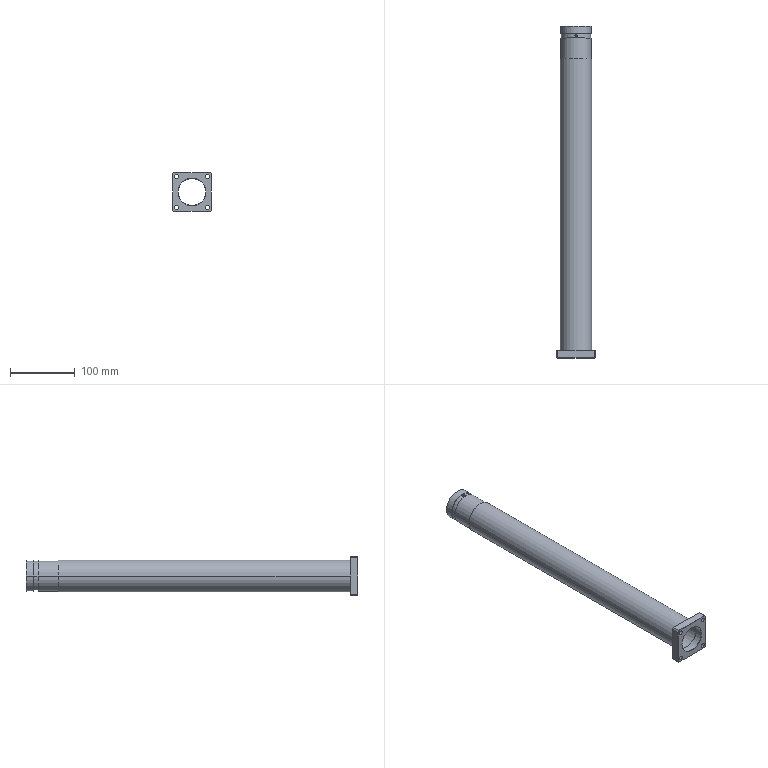Part | NX | 1 solid | 53 faces | box 60 x 512 x 60 mm | volume 225964 mm3 | plane 23 | cylinder 22 | cone 6 | spline 2 | commonest cylinder face diameters 6.5 x8 47 x4 3.3 x2 42 x2 42.8 x2 45 x2